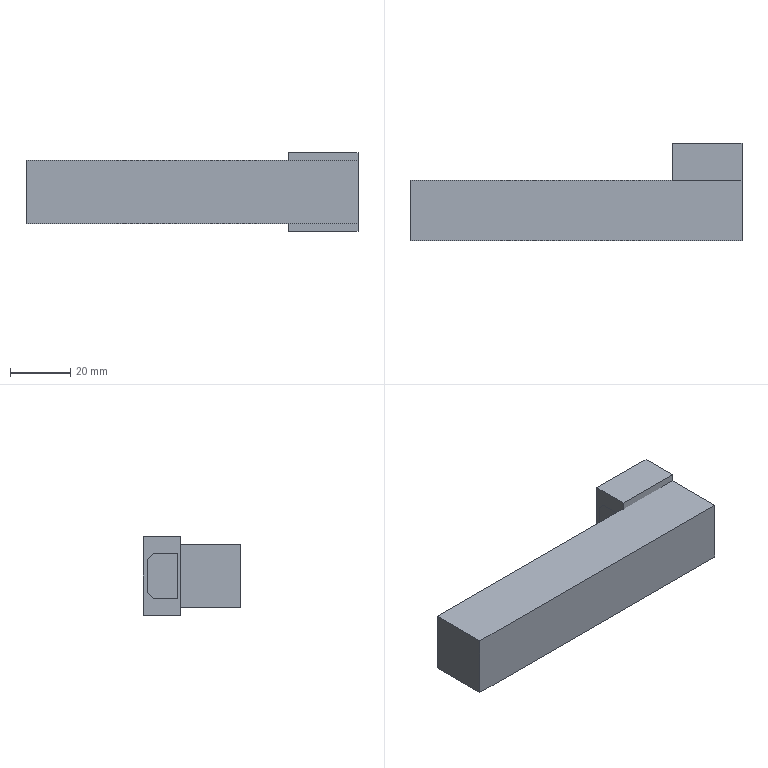NC program | NX | posted with a generic post | part box 110 x 32.2 x 26 mm
Lines 2299 to 4081 of 5595:
(PLANAR_MILL_2_COPY , TOOL : D4J)
N4560 T04 M6
N4562 G54
N4564 G17 G0 G90 X-42.552 Y0.455 S3500 M3
N4566 G43 Z20. H4
N4568 Z-2.067
N4570 G94 G1 Z-4.067 F400.
N4572 G41 X-42.5 Y0.75 D4
N4574 G3 X-43. Y1.25 R0.5
N4576 X-44.25 Y0. R1.25
N4578 X-43. Y-1.25 R1.25
N4580 G1 X22.
N4582 G3 X23.25 Y0. R1.25
N4584 X22. Y1.25 R1.25
N4586 G1 X-43.
N4588 G3 X-43.5 Y0.75 R0.5
N4590 G40
N4592 G1 X-43.448 Y0.455
N4594 X-42.552
N4596 G41 X-42.5 Y0.75
N4598 G3 X-43. Y1.25 R0.5
N4600 X-44.25 Y0. R1.25
N4602 X-43. Y-1.25 R1.25
N4604 G1 X22.
N4606 G3 X23.25 Y0. R1.25
N4608 X22. Y1.25 R1.25
N4610 G1 X-43.
N4612 G3 X-43.5 Y0.75 R0.5
N4614 G1 Y0.559
N4616 G40
N4618 X-43.448 Y0.264
N4620 Z-2.067
N4622 G0 Z20.
N4624 X-42.552 Y0.455
N4626 Z-6.133
N4628 G1 Z-8.133
N4630 G41 X-42.5 Y0.75
N4632 G3 X-43. Y1.25 R0.5
N4634 X-44.25 Y0. R1.25
N4636 X-43. Y-1.25 R1.25
N4638 G1 X22.
N4640 G3 X23.25 Y0. R1.25
N4642 X22. Y1.25 R1.25
N4644 G1 X-43.
N4646 G3 X-43.5 Y0.75 R0.5
N4648 G40
N4650 G1 X-43.448 Y0.455
N4652 X-42.552
N4654 G41 X-42.5 Y0.75
N4656 G3 X-43. Y1.25 R0.5
N4658 X-44.25 Y0. R1.25
N4660 X-43. Y-1.25 R1.25
N4662 G1 X22.
N4664 G3 X23.25 Y0. R1.25
N4666 X22. Y1.25 R1.25
N4668 G1 X-43.
N4670 G3 X-43.5 Y0.75 R0.5
N4672 G1 Y0.559
N4674 G40
N4676 X-43.448 Y0.264
N4678 Z-6.133
N4680 G0 Z20.
N4682 X-42.552 Y0.455
N4684 Z-10.2
N4686 G1 Z-12.2
N4688 G41 X-42.5 Y0.75
N4690 G3 X-43. Y1.25 R0.5
N4692 X-44.25 Y0. R1.25
N4694 X-43. Y-1.25 R1.25
N4696 G1 X22.
N4698 G3 X23.25 Y0. R1.25
N4700 X22. Y1.25 R1.25
N4702 G1 X-43.
N4704 G3 X-43.5 Y0.75 R0.5
N4706 G40
N4708 G1 X-43.448 Y0.455
N4710 X-42.552
N4712 G41 X-42.5 Y0.75
N4714 G3 X-43. Y1.25 R0.5
N4716 X-44.25 Y0. R1.25
N4718 X-43. Y-1.25 R1.25
N4720 G1 X22.
N4722 G3 X23.25 Y0. R1.25
N4724 X22. Y1.25 R1.25
N4726 G1 X-43.
N4728 G3 X-43.5 Y0.75 R0.5
N4730 G1 Y0.559
N4732 G40
N4734 X-43.448 Y0.264
N4736 Z-10.2
N4738 G0 Z20.
(FLOOR_WALL_1_COPY , TOOL : D4J)
N4740 X41. Y-11.44
N4742 Z-5.
N4744 G1 Z-7.
N4746 Y-6.44
N4748 X37.03
N4750 Y6.44
N4752 X44.97
N4754 Y-6.44
N4756 X41.
N4758 Y-3.44
N4760 X40.03
N4762 Y3.44
N4764 X41.97
N4766 Y-3.44
N4768 X41.
N4770 X40.03
N4772 Y-3.41
N4774 X38.03
N4776 Y-11.47
N4778 Z-5.
N4780 G0 Z20.
(PLANAR_MILL_3 , TOOL : D4J)
N4782 X37.174 Y12.425
N4784 Z-4.
N4786 G1 Z-7.
N4788 G41 X37. Y11.44
N4790 Y7.44
N4792 Y-7.44
N4794 Y-11.44
N4796 G40
N4798 X37.174 Y-12.425
N4800 Z-4.
N4802 G0 Z20.
N4804 X44.826
N4806 Z-4.
N4808 G1 Z-7.
N4810 G41 X45. Y-11.44
N4812 Y-7.44
N4814 Y7.44
N4816 Y11.44
N4818 G40
N4820 X44.826 Y12.425
N4822 Z-4.
N4824 G0 Z20.
N4826 M5
(PLANAR_MILL_COPY , TOOL : D16C)
N4828 T01 M6
N4830 G53
N4832 G17 G0 G90 X66. Y-0.06 S2300 M3
N4834 G43 Z20. H1
N4836 Z3.
N4838 G94 G1 Z0. F800.
N4840 X50.
N4842 X-48.06
N4844 X-64.06
N4846 Z3.
N4848 G0 Z20.
N4850 M5
(PLANAR_MILL_4 , TOOL : D4C)
N4852 T03 M6
N4854 G53
N4856 G17 G0 G90 X40.207 Y-0.973 S3500 M3
N4858 G43 Z20. H3
N4860 Z0.2
N4862 G94 G1 X40.724 Y-1.252 Z0.192 F800.
N4864 X41.276 Z0.184
N4866 X41.892 Y-0.92 Z0.174
N4868 X42.243 Y-0.313 Z0.165
N4870 X42.222 Y0.387 Z0.155
N4872 X41.946 Y0.864 Z0.147
N4874 X41.276 Y1.252 Z0.136
N4876 X40.724 Z0.129
N4878 X40.054 Y0.864 Z0.118
N4880 X39.778 Y0.387 Z0.11
N4882 X39.757 Y-0.313 Z0.1
N4884 X40.108 Y-0.92 Z0.09
N4886 X40.724 Y-1.252 Z0.081
N4888 X41.276 Z0.073
N4890 X41.892 Y-0.92 Z0.063
N4892 X42.243 Y-0.313 Z0.053
N4894 X42.222 Y0.387 Z0.044
N4896 X41.946 Y0.864 Z0.036
N4898 X41.276 Y1.252 Z0.025
N4900 X40.724 Z0.017
N4902 X40.054 Y0.864 Z0.007
N4904 X39.778 Y0.387 Z-0.001
N4906 X39.757 Y-0.313 Z-0.011
N4908 X40.108 Y-0.92 Z-0.021
N4910 X40.724 Y-1.252 Z-0.03
N4912 X41.276 Z-0.038
N4914 X41.892 Y-0.92 Z-0.048
N4916 X42.243 Y-0.313 Z-0.058
N4918 X42.222 Y0.387 Z-0.067
N4920 X41.946 Y0.864 Z-0.075
N4922 X41.276 Y1.252 Z-0.086
N4924 X40.724 Z-0.094
N4926 X40.054 Y0.864 Z-0.104
N4928 X39.778 Y0.387 Z-0.112
N4930 X39.757 Y-0.313 Z-0.122
N4932 X40.108 Y-0.92 Z-0.132
N4934 X40.724 Y-1.252 Z-0.141
N4936 X41.276 Z-0.149
N4938 X41.892 Y-0.92 Z-0.159
N4940 X42.243 Y-0.313 Z-0.169
N4942 X42.222 Y0.387 Z-0.179
N4944 X41.946 Y0.864 Z-0.186
N4946 X41.276 Y1.252 Z-0.197
N4948 X40.724 Z-0.205
N4950 X40.054 Y0.864 Z-0.216
N4952 X39.778 Y0.387 Z-0.223
N4954 X39.757 Y-0.313 Z-0.233
N4956 X40.108 Y-0.92 Z-0.243
N4958 X40.724 Y-1.252 Z-0.253
N4960 X41.276 Z-0.26
N4962 X41.892 Y-0.92 Z-0.27
N4964 X42.243 Y-0.313 Z-0.28
N4966 X42.222 Y0.387 Z-0.29
N4968 X41.946 Y0.864 Z-0.297
N4970 X41.276 Y1.252 Z-0.308
N4972 X40.724 Z-0.316
N4974 X40.054 Y0.864 Z-0.327
N4976 X39.778 Y0.387 Z-0.334
N4978 X39.757 Y-0.313 Z-0.344
N4980 X40.108 Y-0.92 Z-0.354
N4982 X40.724 Y-1.252 Z-0.364
N4984 X41.276 Z-0.371
N4986 X41.892 Y-0.92 Z-0.381
N4988 X42.243 Y-0.313 Z-0.391
N4990 X42.222 Y0.387 Z-0.401
N4992 X41.946 Y0.864 Z-0.408
N4994 X41.276 Y1.252 Z-0.419
N4996 X40.724 Z-0.427
N4998 X40.054 Y0.864 Z-0.438
N5000 X39.778 Y0.387 Z-0.445
N5002 X39.757 Y-0.313 Z-0.455
N5004 X40.108 Y-0.92 Z-0.465
N5006 X40.724 Y-1.252 Z-0.475
N5008 X41.276 Z-0.482
N5010 X41.892 Y-0.92 Z-0.492
N5012 X42.243 Y-0.313 Z-0.502
N5014 X42.222 Y0.387 Z-0.512
N5016 X41.946 Y0.864 Z-0.519
N5018 X41.276 Y1.252 Z-0.53
N5020 X40.724 Z-0.538
N5022 X40.054 Y0.864 Z-0.549
N5024 X39.778 Y0.387 Z-0.557
N5026 X39.757 Y-0.313 Z-0.566
N5028 X40.108 Y-0.92 Z-0.576
N5030 X40.724 Y-1.252 Z-0.586
N5032 X41.276 Z-0.594
N5034 X41.892 Y-0.92 Z-0.603
N5036 X42.243 Y-0.313 Z-0.613
N5038 X42.222 Y0.387 Z-0.623
N5040 X41.946 Y0.864 Z-0.631
N5042 X41.276 Y1.252 Z-0.641
N5044 X40.724 Z-0.649
N5046 X40.054 Y0.864 Z-0.66
N5048 X39.778 Y0.387 Z-0.668
N5050 X39.757 Y-0.313 Z-0.677
N5052 X40.108 Y-0.92 Z-0.687
N5054 X40.724 Y-1.252 Z-0.697
N5056 X41.276 Z-0.705
N5058 X41.892 Y-0.92 Z-0.714
N5060 X42.243 Y-0.313 Z-0.724
N5062 X42.222 Y0.387 Z-0.734
N5064 X41.946 Y0.864 Z-0.742
N5066 X41.276 Y1.252 Z-0.752
N5068 X40.724 Z-0.76
N5070 X40.054 Y0.864 Z-0.771
N5072 X39.778 Y0.387 Z-0.779
N5074 X39.757 Y-0.313 Z-0.788
N5076 X40.108 Y-0.92 Z-0.798
N5078 X40.724 Y-1.252 Z-0.808
N5080 X41.276 Z-0.816
N5082 X41.892 Y-0.92 Z-0.826
N5084 X42.243 Y-0.313 Z-0.835
N5086 X42.222 Y0.387 Z-0.845
N5088 X41.946 Y0.864 Z-0.853
N5090 X41.276 Y1.252 Z-0.864
N5092 X40.724 Z-0.871
N5094 X40.054 Y0.864 Z-0.882
N5096 X39.778 Y0.387 Z-0.89
N5098 X39.757 Y-0.313 Z-0.9
N5100 X40.108 Y-0.92 Z-0.909
N5102 X40.724 Y-1.252 Z-0.919
N5104 X41.276 Z-0.927
N5106 X41.892 Y-0.92 Z-0.937
N5108 X42.243 Y-0.313 Z-0.946
N5110 X42.222 Y0.387 Z-0.956
N5112 X41.946 Y0.864 Z-0.964
N5114 X41.276 Y1.252 Z-0.975
N5116 X40.724 Z-0.982
N5118 X40.054 Y0.864 Z-0.993
N5120 X39.778 Y0.387 Z-1.001
N5122 X39.757 Y-0.313 Z-1.011
N5124 X40.108 Y-0.92 Z-1.02
N5126 X40.724 Y-1.252 Z-1.03
N5128 X41.276 Z-1.038
N5130 X41.892 Y-0.92 Z-1.048
N5132 X42.243 Y-0.313 Z-1.057
N5134 X42.222 Y0.387 Z-1.067
N5136 X41.946 Y0.864 Z-1.075
N5138 X41.276 Y1.252 Z-1.086
N5140 X40.724 Z-1.093
N5142 X40.054 Y0.864 Z-1.104
N5144 X39.778 Y0.387 Z-1.112
N5146 X39.757 Y-0.313 Z-1.122
N5148 X40.108 Y-0.92 Z-1.132
N5150 X40.724 Y-1.252 Z-1.141
N5152 X41.276 Z-1.149
N5154 X41.892 Y-0.92 Z-1.159
N5156 X42.243 Y-0.313 Z-1.169
N5158 X42.222 Y0.387 Z-1.178
N5160 X41.946 Y0.864 Z-1.186
N5162 X41.276 Y1.252 Z-1.197
N5164 X40.724 Z-1.205
N5166 X40.054 Y0.864 Z-1.215
N5168 X39.778 Y0.387 Z-1.223
N5170 X39.757 Y-0.313 Z-1.233
N5172 X40.108 Y-0.92 Z-1.243
N5174 X40.724 Y-1.252 Z-1.252
N5176 X41.276 Z-1.26
N5178 X41.892 Y-0.92 Z-1.27
N5180 X42.243 Y-0.313 Z-1.28
N5182 X42.222 Y0.387 Z-1.289
N5184 X41.946 Y0.864 Z-1.297
N5186 X41.276 Y1.252 Z-1.308
N5188 X40.724 Z-1.316
N5190 X40.054 Y0.864 Z-1.326
N5192 X39.778 Y0.387 Z-1.334
N5194 X39.757 Y-0.313 Z-1.344
N5196 X40.108 Y-0.92 Z-1.354
N5198 X40.724 Y-1.252 Z-1.363
N5200 X41.276 Z-1.371
N5202 X41.892 Y-0.92 Z-1.381
N5204 X42.243 Y-0.313 Z-1.391
N5206 X42.222 Y0.387 Z-1.401
N5208 X41.946 Y0.864 Z-1.408
N5210 X41.276 Y1.252 Z-1.419
N5212 X40.724 Z-1.427
N5214 X40.054 Y0.864 Z-1.438
N5216 X39.778 Y0.387 Z-1.445
N5218 X39.757 Y-0.313 Z-1.455
N5220 X40.108 Y-0.92 Z-1.465
N5222 X40.724 Y-1.252 Z-1.475
N5224 X41.276 Z-1.482
N5226 X41.892 Y-0.92 Z-1.492
N5228 X42.243 Y-0.313 Z-1.502
N5230 X42.222 Y0.387 Z-1.512
N5232 X41.946 Y0.864 Z-1.519
N5234 X41.276 Y1.252 Z-1.53
N5236 X40.724 Z-1.538
N5238 X40.054 Y0.864 Z-1.549
N5240 X39.778 Y0.387 Z-1.556
N5242 X39.757 Y-0.313 Z-1.566
N5244 X40.108 Y-0.92 Z-1.576
N5246 X40.724 Y-1.252 Z-1.586
N5248 X41.276 Z-1.593
N5250 X41.892 Y-0.92 Z-1.603
N5252 X42.243 Y-0.313 Z-1.613
N5254 X42.222 Y0.387 Z-1.623
N5256 X41.946 Y0.864 Z-1.63
N5258 X41.276 Y1.252 Z-1.641
N5260 X40.724 Z-1.649
N5262 X40.054 Y0.864 Z-1.66
N5264 X39.778 Y0.387 Z-1.667
N5266 X39.757 Y-0.313 Z-1.677
N5268 X40.108 Y-0.92 Z-1.687
N5270 X40.724 Y-1.252 Z-1.697
N5272 X41.276 Z-1.704
N5274 X41.892 Y-0.92 Z-1.714
N5276 X42.243 Y-0.313 Z-1.724
N5278 X42.222 Y0.387 Z-1.734
N5280 X41.946 Y0.864 Z-1.742
N5282 X41.276 Y1.252 Z-1.752
N5284 X40.724 Z-1.76
N5286 X40.054 Y0.864 Z-1.771
N5288 X39.778 Y0.387 Z-1.779
N5290 X39.757 Y-0.313 Z-1.788
N5292 X40.108 Y-0.92 Z-1.798
N5294 X40.724 Y-1.252 Z-1.808
N5296 X41.276 Z-1.816
N5298 X41.892 Y-0.92 Z-1.825
N5300 X42.243 Y-0.313 Z-1.835
N5302 X42.222 Y0.387 Z-1.845
N5304 X41.946 Y0.864 Z-1.853
N5306 X41.276 Y1.252 Z-1.863
N5308 X40.724 Z-1.871
N5310 X40.054 Y0.864 Z-1.882
N5312 X39.778 Y0.387 Z-1.89
N5314 X39.757 Y-0.313 Z-1.899
N5316 X40.108 Y-0.92 Z-1.909
N5318 X40.724 Y-1.252 Z-1.919
N5320 X41.276 Z-1.927
N5322 X41.892 Y-0.92 Z-1.936
N5324 X42.243 Y-0.313 Z-1.946
N5326 X42.222 Y0.387 Z-1.956
N5328 X41.946 Y0.864 Z-1.964
N5330 X41.276 Y1.252 Z-1.974
N5332 X40.724 Z-1.982
N5334 X40.054 Y0.864 Z-1.993
N5336 X39.778 Y0.387 Z-2.001
N5338 X39.757 Y-0.313 Z-2.01
N5340 X40.108 Y-0.92 Z-2.02
N5342 X40.724 Y-1.252 Z-2.03
N5344 X41.276 Z-2.038
N5346 X41.892 Y-0.92 Z-2.048
N5348 X42.243 Y-0.313 Z-2.057
N5350 X42.222 Y0.387 Z-2.067
N5352 X41.946 Y0.864 Z-2.075
N5354 X41.276 Y1.252 Z-2.086
N5356 X40.724 Z-2.093
N5358 X40.054 Y0.864 Z-2.104
N5360 X39.778 Y0.387 Z-2.112
N5362 X39.757 Y-0.313 Z-2.122
N5364 X40.108 Y-0.92 Z-2.131
N5366 X40.724 Y-1.252 Z-2.141
N5368 X41.276 Z-2.149
N5370 X41.892 Y-0.92 Z-2.159
N5372 X42.243 Y-0.313 Z-2.168
N5374 X42.222 Y0.387 Z-2.178
N5376 X41.946 Y0.864 Z-2.186
N5378 X41.276 Y1.252 Z-2.197
N5380 X40.724 Z-2.204
N5382 X40.054 Y0.864 Z-2.215
N5384 X39.778 Y0.387 Z-2.223
N5386 X39.757 Y-0.313 Z-2.233
N5388 X40.108 Y-0.92 Z-2.242
N5390 X40.724 Y-1.252 Z-2.252
N5392 X41.276 Z-2.26
N5394 X41.892 Y-0.92 Z-2.27
N5396 X42.243 Y-0.313 Z-2.279
N5398 X42.222 Y0.387 Z-2.289
N5400 X41.946 Y0.864 Z-2.297
N5402 X41.276 Y1.252 Z-2.308
N5404 X40.724 Z-2.315
N5406 X40.054 Y0.864 Z-2.326
N5408 X39.778 Y0.387 Z-2.334
N5410 X39.757 Y-0.313 Z-2.344
N5412 X40.108 Y-0.92 Z-2.354
N5414 X40.724 Y-1.252 Z-2.363
N5416 X41.276 Z-2.371
N5418 X41.892 Y-0.92 Z-2.381
N5420 X42.243 Y-0.313 Z-2.391
N5422 X42.222 Y0.387 Z-2.4
N5424 X41.946 Y0.864 Z-2.408
N5426 X41.276 Y1.252 Z-2.419
N5428 X40.724 Z-2.427
N5430 X40.054 Y0.864 Z-2.437
N5432 X39.778 Y0.387 Z-2.445
N5434 X39.757 Y-0.313 Z-2.455
N5436 X40.108 Y-0.92 Z-2.465
N5438 X40.724 Y-1.252 Z-2.474
N5440 X41.276 Z-2.482
N5442 X41.892 Y-0.92 Z-2.492
N5444 X42.243 Y-0.313 Z-2.502
N5446 X42.222 Y0.387 Z-2.511
N5448 X41.946 Y0.864 Z-2.519
N5450 X41.276 Y1.252 Z-2.53
N5452 X40.724 Z-2.538
N5454 X40.054 Y0.864 Z-2.548
N5456 X39.778 Y0.387 Z-2.556
N5458 X39.757 Y-0.313 Z-2.566
N5460 X40.108 Y-0.92 Z-2.576
N5462 X40.724 Y-1.252 Z-2.586
N5464 X41.276 Z-2.593
N5466 X41.892 Y-0.92 Z-2.603
N5468 X42.243 Y-0.313 Z-2.613
N5470 X42.222 Y0.387 Z-2.623
N5472 X41.946 Y0.864 Z-2.63
N5474 X41.276 Y1.252 Z-2.641
N5476 X40.724 Z-2.649
N5478 X40.054 Y0.864 Z-2.66
N5480 X39.778 Y0.387 Z-2.667
N5482 X39.757 Y-0.313 Z-2.677
N5484 X40.108 Y-0.92 Z-2.687
N5486 X40.724 Y-1.252 Z-2.697
N5488 X41.276 Z-2.704
N5490 X41.892 Y-0.92 Z-2.714
N5492 X42.243 Y-0.313 Z-2.724
N5494 X42.222 Y0.387 Z-2.734
N5496 X41.946 Y0.864 Z-2.741
N5498 X41.276 Y1.252 Z-2.752
N5500 X40.724 Z-2.76
N5502 X40.054 Y0.864 Z-2.771
N5504 X39.778 Y0.387 Z-2.778
N5506 X39.757 Y-0.313 Z-2.788
N5508 X40.108 Y-0.92 Z-2.798
N5510 X40.724 Y-1.252 Z-2.808
N5512 X41.276 Z-2.815
N5514 X41.892 Y-0.92 Z-2.825
N5516 X42.243 Y-0.313 Z-2.835
N5518 X42.222 Y0.387 Z-2.845
N5520 X41.946 Y0.864 Z-2.852
N5522 X41.276 Y1.252 Z-2.863
N5524 X40.724 Z-2.871
N5526 X40.054 Y0.864 Z-2.882
N5528 X39.778 Y0.387 Z-2.889
N5530 X39.757 Y-0.313 Z-2.899
N5532 X40.108 Y-0.92 Z-2.909
N5534 X40.724 Y-1.252 Z-2.919
N5536 X41.276 Z-2.926
N5538 X41.892 Y-0.92 Z-2.936
N5540 X42.243 Y-0.313 Z-2.946
N5542 X42.222 Y0.387 Z-2.956
N5544 X41.946 Y0.864 Z-2.964
N5546 X41.276 Y1.252 Z-2.974
N5548 X40.724 Z-2.982
N5550 X40.054 Y0.864 Z-2.993
N5552 X39.778 Y0.387 Z-3.001
N5554 X39.757 Y-0.313 Z-3.01
N5556 X40.108 Y-0.92 Z-3.02
N5558 X40.724 Y-1.252 Z-3.03
N5560 X41.276 Z-3.038
N5562 X41.892 Y-0.92 Z-3.047
N5564 X42.243 Y-0.313 Z-3.057
N5566 X42.222 Y0.387 Z-3.067
N5568 X41.946 Y0.864 Z-3.075
N5570 X41.276 Y1.252 Z-3.085
N5572 X40.724 Z-3.093
N5574 X40.054 Y0.864 Z-3.104
N5576 X39.778 Y0.387 Z-3.112
N5578 X39.757 Y-0.313 Z-3.121
N5580 X40.108 Y-0.92 Z-3.131
N5582 X40.724 Y-1.252 Z-3.141
N5584 X41.276 Z-3.149
N5586 X41.892 Y-0.92 Z-3.158
N5588 X42.243 Y-0.313 Z-3.168
N5590 X42.222 Y0.387 Z-3.178
N5592 X41.946 Y0.864 Z-3.186
N5594 X41.276 Y1.252 Z-3.197
N5596 X40.724 Z-3.204
N5598 X40.054 Y0.864 Z-3.215
N5600 X39.778 Y0.387 Z-3.223
N5602 X39.757 Y-0.313 Z-3.232
N5604 X40.108 Y-0.92 Z-3.242
N5606 X40.724 Y-1.252 Z-3.252
N5608 X41.276 Z-3.26
N5610 X41.892 Y-0.92 Z-3.27
N5612 X42.243 Y-0.313 Z-3.279
N5614 X42.222 Y0.387 Z-3.289
N5616 X41.946 Y0.864 Z-3.297
N5618 X41.276 Y1.252 Z-3.308
N5620 X40.724 Z-3.315
N5622 X40.054 Y0.864 Z-3.326
N5624 X39.778 Y0.387 Z-3.334
N5626 X39.757 Y-0.313 Z-3.344
N5628 X40.108 Y-0.92 Z-3.353
N5630 X40.724 Y-1.252 Z-3.363
N5632 X41.276 Z-3.371
N5634 X41.892 Y-0.92 Z-3.381
N5636 X42.243 Y-0.313 Z-3.39
N5638 X42.222 Y0.387 Z-3.4
N5640 X41.946 Y0.864 Z-3.408
N5642 X41.276 Y1.252 Z-3.419
N5644 X40.724 Z-3.426
N5646 X40.054 Y0.864 Z-3.437
N5648 X39.778 Y0.387 Z-3.445
N5650 X39.757 Y-0.313 Z-3.455
N5652 X40.108 Y-0.92 Z-3.464
N5654 X40.724 Y-1.252 Z-3.474
N5656 X41.276 Z-3.482
N5658 X41.892 Y-0.92 Z-3.492
N5660 X42.243 Y-0.313 Z-3.501
N5662 X42.222 Y0.387 Z-3.511
N5664 X41.946 Y0.864 Z-3.519
N5666 X41.276 Y1.252 Z-3.53
N5668 X40.724 Z-3.537
N5670 X40.054 Y0.864 Z-3.548
N5672 X39.778 Y0.387 Z-3.556
N5674 X39.757 Y-0.313 Z-3.566
N5676 X40.108 Y-0.92 Z-3.576
N5678 X40.724 Y-1.252 Z-3.585
N5680 X41.276 Z-3.593
N5682 X41.892 Y-0.92 Z-3.603
N5684 X42.243 Y-0.313 Z-3.613
N5686 X42.222 Y0.387 Z-3.622
N5688 X41.946 Y0.864 Z-3.63
N5690 X41.276 Y1.252 Z-3.641
N5692 X40.724 Z-3.649
N5694 X40.054 Y0.864 Z-3.659
N5696 X39.778 Y0.387 Z-3.667
N5698 X39.757 Y-0.313 Z-3.677
N5700 X40.108 Y-0.92 Z-3.687
N5702 X40.724 Y-1.252 Z-3.696
N5704 X41.276 Z-3.704
N5706 X41.892 Y-0.92 Z-3.714
N5708 X42.243 Y-0.313 Z-3.724
N5710 X42.222 Y0.387 Z-3.733
N5712 X41.946 Y0.864 Z-3.741
N5714 X41.276 Y1.252 Z-3.752
N5716 X40.724 Z-3.76
N5718 X40.054 Y0.864 Z-3.77
N5720 X39.778 Y0.387 Z-3.778
N5722 X39.757 Y-0.313 Z-3.788
N5724 X40.108 Y-0.92 Z-3.798
N5726 X40.724 Y-1.252 Z-3.808
N5728 X41.276 Z-3.815
N5730 X41.892 Y-0.92 Z-3.825
N5732 X42.243 Y-0.313 Z-3.835
N5734 X42.222 Y0.387 Z-3.845
N5736 X41.946 Y0.864 Z-3.852
N5738 X41.276 Y1.252 Z-3.863
N5740 X40.724 Z-3.871
N5742 X40.054 Y0.864 Z-3.882
N5744 X39.778 Y0.387 Z-3.889
N5746 X39.757 Y-0.313 Z-3.899
N5748 X40.108 Y-0.92 Z-3.909
N5750 X40.724 Y-1.252 Z-3.919
N5752 X41.276 Z-3.926
N5754 X41.892 Y-0.92 Z-3.936
N5756 X42.243 Y-0.313 Z-3.946
N5758 X42.222 Y0.387 Z-3.956
N5760 X41.946 Y0.864 Z-3.963
N5762 X41.276 Y1.252 Z-3.974
N5764 X40.724 Z-3.982
N5766 X40.054 Y0.864 Z-3.993
N5768 X39.778 Y0.387 Z-4.
N5770 X39.757 Y-0.313 Z-4.01
N5772 X40.108 Y-0.92 Z-4.02
N5774 X40.724 Y-1.252 Z-4.03
N5776 X41.276 Z-4.037
N5778 X41.892 Y-0.92 Z-4.047
N5780 X42.243 Y-0.313 Z-4.057
N5782 X42.222 Y0.387 Z-4.067
N5784 X41.946 Y0.864 Z-4.074
N5786 X41.276 Y1.252 Z-4.085
N5788 X40.724 Z-4.093
N5790 X40.054 Y0.864 Z-4.104
N5792 X39.778 Y0.387 Z-4.111
N5794 X39.757 Y-0.313 Z-4.121
N5796 X40.108 Y-0.92 Z-4.131
N5798 X40.724 Y-1.252 Z-4.141
N5800 X41.276 Z-4.148
N5802 X41.892 Y-0.92 Z-4.158
N5804 X42.243 Y-0.313 Z-4.168
N5806 X42.222 Y0.387 Z-4.178
N5808 X41.946 Y0.864 Z-4.186
N5810 X41.276 Y1.252 Z-4.196
N5812 X40.724 Z-4.204
N5814 X40.054 Y0.864 Z-4.215
N5816 X39.778 Y0.387 Z-4.223
N5818 X39.757 Y-0.313 Z-4.232
N5820 X40.108 Y-0.92 Z-4.242
N5822 X40.724 Y-1.252 Z-4.252
N5824 X41.276 Z-4.26
N5826 X41.892 Y-0.92 Z-4.269
N5828 X42.243 Y-0.313 Z-4.279
N5830 X42.222 Y0.387 Z-4.289
N5832 X41.946 Y0.864 Z-4.297
N5834 X41.276 Y1.252 Z-4.307
N5836 X40.724 Z-4.315
N5838 X40.054 Y0.864 Z-4.326
N5840 X39.778 Y0.387 Z-4.334
N5842 X39.757 Y-0.313 Z-4.343
N5844 X40.108 Y-0.92 Z-4.353
N5846 X40.724 Y-1.252 Z-4.363
N5848 X41.276 Z-4.371
N5850 X41.892 Y-0.92 Z-4.38
N5852 X42.243 Y-0.313 Z-4.39
N5854 X42.222 Y0.387 Z-4.4
N5856 X41.946 Y0.864 Z-4.408
N5858 X41.276 Y1.252 Z-4.419
N5860 X40.724 Z-4.426
N5862 X40.054 Y0.864 Z-4.437
N5864 X39.778 Y0.387 Z-4.445
N5866 X39.757 Y-0.313 Z-4.454
N5868 X40.108 Y-0.92 Z-4.464
N5870 X40.724 Y-1.252 Z-4.474
N5872 X41.276 Z-4.482
N5874 X41.892 Y-0.92 Z-4.492
N5876 X42.243 Y-0.313 Z-4.501
N5878 X42.222 Y0.387 Z-4.511
N5880 X41.946 Y0.864 Z-4.519
N5882 X41.276 Y1.252 Z-4.53
N5884 X40.724 Z-4.537
N5886 X40.054 Y0.864 Z-4.548
N5888 X39.778 Y0.387 Z-4.556
N5890 X39.757 Y-0.313 Z-4.566
N5892 X40.108 Y-0.92 Z-4.575
N5894 X40.724 Y-1.252 Z-4.585
N5896 X41.276 Z-4.593
N5898 X41.892 Y-0.92 Z-4.603
N5900 X42.243 Y-0.313 Z-4.612
N5902 X42.222 Y0.387 Z-4.622
N5904 X41.946 Y0.864 Z-4.63
N5906 X41.276 Y1.252 Z-4.641
N5908 X40.724 Z-4.648
N5910 X40.054 Y0.864 Z-4.659
N5912 X39.778 Y0.387 Z-4.667
N5914 X39.757 Y-0.313 Z-4.677
N5916 X40.108 Y-0.92 Z-4.686
N5918 X40.724 Y-1.252 Z-4.696
N5920 X41.276 Z-4.704
N5922 X41.892 Y-0.92 Z-4.714
N5924 X42.243 Y-0.313 Z-4.723
N5926 X42.222 Y0.387 Z-4.733
N5928 X41.946 Y0.864 Z-4.741
N5930 X41.276 Y1.252 Z-4.752
N5932 X40.724 Z-4.759
N5934 X40.054 Y0.864 Z-4.77
N5936 X39.778 Y0.387 Z-4.778
N5938 X39.757 Y-0.313 Z-4.788
N5940 X40.108 Y-0.92 Z-4.798
N5942 X40.724 Y-1.252 Z-4.807
N5944 X41.276 Z-4.815
N5946 X41.892 Y-0.92 Z-4.825
N5948 X42.243 Y-0.313 Z-4.835
N5950 X42.222 Y0.387 Z-4.844
N5952 X41.946 Y0.864 Z-4.852
N5954 X41.276 Y1.252 Z-4.863
N5956 X40.724 Z-4.871
N5958 X40.054 Y0.864 Z-4.881
N5960 X39.778 Y0.387 Z-4.889
N5962 X39.757 Y-0.313 Z-4.899
N5964 X40.108 Y-0.92 Z-4.909
N5966 X40.724 Y-1.252 Z-4.918
N5968 X41.276 Z-4.926
N5970 X41.892 Y-0.92 Z-4.936
N5972 X42.243 Y-0.313 Z-4.946
N5974 X42.222 Y0.387 Z-4.955
N5976 X41.946 Y0.864 Z-4.963
N5978 X41.276 Y1.252 Z-4.974
N5980 X40.724 Z-4.982
N5982 X40.054 Y0.864 Z-4.992
N5984 X39.778 Y0.387 Z-5.
N5986 X39.757 Y-0.313 Z-5.01
N5988 X40.108 Y-0.92 Z-5.02
N5990 X40.724 Y-1.252 Z-5.03
N5992 X41.276 Z-5.037
N5994 X41.892 Y-0.92 Z-5.047
N5996 X42.243 Y-0.313 Z-5.057
N5998 X42.222 Y0.387 Z-5.067
N6000 X41.946 Y0.864 Z-5.074
N6002 X41.276 Y1.252 Z-5.085
N6004 X40.724 Z-5.093
N6006 X40.054 Y0.864 Z-5.104
N6008 X39.778 Y0.387 Z-5.111
N6010 X39.757 Y-0.313 Z-5.121
N6012 X40.108 Y-0.92 Z-5.131
N6014 X40.724 Y-1.252 Z-5.141
N6016 X41.276 Z-5.148
N6018 X41.892 Y-0.92 Z-5.158
N6020 X42.243 Y-0.313 Z-5.168
N6022 X42.222 Y0.387 Z-5.178
N6024 X41.946 Y0.864 Z-5.185
N6026 X41.276 Y1.252 Z-5.196
N6028 X41. Z-5.2
N6030 G3 X39.749 Y0. R1.252
N6032 X41. Y1.252 R-1.252
N6034 G1 Z-5.
N6036 G0 Z20.
N6038 M5
(PLANAR_MILL_5 , TOOL : D4DJ)
N6040 T05 M6
N6042 G53
N6044 G17 G0 G90 X23. Y0.75 S3000 M3
N6046 G43 Z20. H5
N6048 Z1.
N6050 G94 G1 Z-1. F1000.
N6052 Y1.25
N6054 G3 X22. Y2.25 R1.
N6056 G1 X-43.
N6058 G3 X-45.25 Y0. R2.25
N6060 X-43. Y-2.25 R2.25
N6062 G1 X22.
N6064 G3 X24.25 Y0. R2.25
N6066 X22. Y2.25 R2.25
N6068 X21. Y1.25 R1.
N6070 G1 Z1.
N6072 G0 Z20.
N6074 X40. Y-0.752
N6076 Z1.
N6078 G1 Z-1.
N6080 Y-1.252
N6082 G3 X41. Y-2.252 R1.
N6084 X43.252 Y0. R2.252
N6086 X41. Y-2.252 R-2.252
N6088 X42. Y-1.252 R1.
N6090 G1 Y-0.752
N6092 Z1.
N6094 G0 Z20.
(PLANAR_MILL_5_COPY , TOOL : D4DJ)
N6096 X52. Y-6.44
N6098 Z1.
N6100 G1 Z-1.
N6102 G3 X51. Y-7.44 R1.
N6104 G2 X50. Y-8.44 R1.
N6106 G1 X-48.06
N6108 G2 X-48.767 Y-8.147 R1.
N6110 G1 X-50.707 Y-6.207
N6112 G2 X-51. Y-5.5 R1.
N6114 G1 Y5.5
N6116 G2 X-50.707 Y6.207 R1.
N6118 G1 X-48.767 Y8.147
N6120 G2 X-48.06 Y8.44 R1.
N6122 G1 X50.
N6124 G2 X51. Y7.44 R1.
N6126 G1 Y-7.44
N6128 G3 X52. Y-8.44 R1.
N6130 G1 Z1.
N6132 G0 Z20.
N6134 M5
(PLANAR_MILL_6 , TOOL : D16C)
N6136 T01 M6
N6138 G54
N6140 G17 G0 G90 X23.5 Y-1. S2300 M3
N6142 G43 Z20. H1
N6144 Z3.
N6146 G94 G1 Z0. F600.
N6148 X7.5
N6150 X-7.5
N6152 X-23.5
N6154 Z3.
N6156 G0 Z20.
(ADAPTIVE_MILLING_1 , TOOL : D16C)
N6158 X25.701 Y14.017 S3500
N6160 Z-16.
N6162 G1 X25.572 Y13.941 Z-16.937 F1500.
N6164 X25.442 Y13.866 Z-17.308
N6166 X25.312 Y13.791 Z-17.58
N6168 X25.182 Y13.716 Z-17.8
N6170 X25.053 Y13.64 Z-17.984
N6172 X24.923 Y13.565 Z-18.142
N6174 X24.793 Y13.49 Z-18.28
N6176 X24.663 Y13.414 Z-18.4
N6178 X24.534 Y13.339 Z-18.505
N6180 X24.404 Y13.264 Z-18.598
N6182 X24.274 Y13.189 Z-18.679
N6184 X24.144 Y13.113 Z-18.75
N6186 X24.015 Y13.038 Z-18.81
N6188 X23.885 Y12.963 Z-18.862
N6190 X23.755 Y12.888 Z-18.905
N6192 X23.625 Y12.812 Z-18.939
N6194 X23.496 Y12.737 Z-18.966
N6196 X23.366 Y12.662 Z-18.985
N6198 X23.236 Y12.586 Z-18.996
N6200 X23.106 Y12.511 Z-19.
N6202 X20.932 Y11.25
N6204 G3 X20.154 Y9.558 R1.616
N6206 G2 X20.587 Y6.395 R12.497
N6208 X20.675 Y-4.516 R227.945
N6210 X17.038 Y-11.021 R8.943
N6212 X11.305 Y-13.391 R13.202
N6214 X5.03 Y-13.862 R39.811
N6216 X-11.22 Y-13.882 R893.255
N6218 X-17.72 Y-10.352 R8.92
N6220 X-20.183 Y-4.531 R13.112
N6222 X-20.662 Y1.782 R39.494
N6224 X-20.615 Y5.004 R26.234
N6226 X-16.75 Y11.211 R9.081
N6228 X-10.952 Y13.446 R13.654
N6230 X-4.522 Y13.869 R44.518
N6232 X10.89 Y13.887 R908.336
N6234 X17.333 Y10.399 R8.956
N6236 X19.838 Y4.636 R13.087
N6238 X20.355 Y-1.635 R37.456
N6240 X15.482 Y-10.823 R10.52
N6242 X9.25 Y-13.099 R15.678
N6244 X2.484 Y-13.559 R48.53
N6246 X-9.328 Y-13.581 R647.832
N6248 X-17.727 Y-8.531 R10.619
N6250 X-19.903 Y-2.422 R15.875
N6252 X-20.265 Y2.77 R27.224
N6254 X-15.482 Y10.79 R10.489
N6256 X-9.331 Y13.078 R15.536
N6258 X-2.604 Y13.557 R46.731
N6260 X9.021 Y13.579 R470.728
N6262 X17.411 Y8.504 R10.671
N6264 X19.617 Y2.24 R16.079
N6266 X19.772 Y-2.39 R15.803
N6268 X14.307 Y-10.534 R11.441
N6270 X7.754 Y-12.789 R17.309
N6272 X0.424 Y-13.259 R55.185
N6274 X-7.895 Y-13.267 R209.836
N6276 X-17.59 Y-7.136 R11.748
N6278 X-19.73 Y1.282 R17.546
N6280 X-14.601 Y10.293 R11.198
N6282 X-11.667 Y11.8 R16.552
N6284 G1 X-11.131 Y12.129
N6286 G2 X-8.565 Y12.931 R9.231
N6288 X2.366 Y13.289 R134.099
N6290 X7.728 Y13.255 R103.637
N6292 X17.216 Y7.222 R11.768
N6294 X19.241 Y-0.563 R14.922
N6296 X13.92 Y-9.812 R11.696
N6298 X9.721 Y-11.779 R16.539
N6300 G1 X9.131 Y-12.129
N6302 G2 X6.75 Y-12.902 R9.316
N6304 G1 X5.499 Y-13.
N6306 G2 X-6.213 Y-12.982 R869.141
N6308 X-14.742 Y-9.531 R12.672
N6310 X-19.028 Y0.004 R14.26
N6312 X-14.794 Y9.079 R11.396
N6314 G1 X-13.81 Y9.892
N6316 X-13.156 Y10.658
N6318 G2 X-11.131 Y12.129 R9.312
N6320 X-8.75 Y12.902 R9.316
N6322 G1 X-7.499 Y13.
N6324 X7.501
N6326 G2 X9.973 Y12.608 R9.319
N6328 X14.326 Y9.824 R11.906
N6330 X18.472 Y1.181 R13.654
N6332 X13.843 Y-8.861 R11.64
N6334 X11.294 Y-10.534 R31.864
N6336 G1 X10.201 Y-11.473
N6338 X9.594 Y-11.845
N6340 G3 X9.623 Y-14.591 R1.6
N6342 X10.785 Y-14.777 Z-18.962 R1.701
N6344 G1 X12.755 Y-14.523 Z-18.9
N6346 X15.598 Y-14.158 F15000.
N6348 G3 X16.525 Y-13.702 R1.604
N6350 G1 X17.433 Y-12.8
N6352 X18.327 Y-11.885
N6354 G3 X20.323 Y-9.147 R14.598
N6356 G1 X22.282 Y-5.674
N6358 G3 X23.552 Y-1.467 R10.091
N6360 X23.365 Y1.977 R12.707
N6362 G1 X22.529 Y6.31
N6364 G3 X20.009 Y11.642 R11.87
N6366 G1 X18.065 Y13.985
N6368 G3 X17.006 Y14.554 R1.602
N6370 G1 X14.35 Y14.842
N6372 X13.198 Y14.972 Z-18.936 F1500.
N6374 X12.045 Y15.087 Z-18.973
N6376 G3 X11.206 Y14.898 Z-19. R1.602
N6378 X11.133 Y12.127 R1.6
N6380 G2 X13.98 Y9.758 R9.314
N6382 X17.296 Y3.876 R15.158
N6384 X14.558 Y-7.092 R11.557
N6386 G3 X13.156 Y-8.657 R27.808
N6388 G1 X11.194 Y-10.619
N6390 G3 X12.198 Y-13.346 R1.6
N6392 X13.094 Y-13.162 Z-18.971 R1.762
N6394 G1 X15.175 Y-12.271 Z-18.9
N6396 X17.669 Y-11.203 F15000.
N6398 G3 X18.37 Y-10.619 R1.608
N6400 G1 X19.366 Y-9.131
N6402 X20.348 Y-7.633
N6404 G3 X22.389 Y-2.737 R16.864
N6406 G1 X22.57 Y-1.984
N6408 X22.741 Y-1.229
N6410 G3 X22.152 Y5.837 R12.944
N6412 G1 X20.334 Y10.656
N6414 G3 X19.378 Y11.597 R1.601
N6416 G1 X16.826 Y12.514
N6418 X15.827 Y12.877 Z-18.933 F1500.
N6420 X14.823 Y13.228 Z-18.967
N6422 G3 X13.782 Y13.181 Z-19. R1.6
N6424 X13.158 Y10.656 R1.6
N6426 G2 X14.629 Y8.631 R9.316
N6428 X16.794 Y3.269 R15.121
N6430 X15.338 Y-4.694 R12.059
N6432 G3 X15.108 Y-5.473 R4.152
N6434 G2 X13.947 Y-7.732 R9.154
N6436 G3 X15.781 Y-10.247 R1.6
N6438 X16.317 Y-9.892 Z-18.98 R1.951
N6440 G1 X18.261 Y-8.252 Z-18.9
N6442 X20.479 Y-6.382 F15000.
N6444 G3 X20.879 Y-5.874 R1.629
N6446 G1 X21.414 Y-4.811
N6448 X21.933 Y-3.74
N6450 G3 X22.422 Y-0.33 R6.63
N6452 G1 X21.56 Y6.774
N6454 G3 X20.879 Y7.899 R1.601
N6456 G1 X18.612 Y9.46
N6458 X16.938 Y10.607 Z-18.964 F1500.
N6460 G3 X15.824 Y10.818 Z-19. R1.6
N6462 X14.629 Y8.631 R1.6
N6464 G2 X16.108 Y4.093 R20.905
N6466 X15.715 Y-2.102 R13.799
N6468 G3 X15.5 Y-3.001 R9.216
N6470 G1 X15.401 Y-4.253
N6472 X15.226 Y-4.982
N6474 G3 X17.181 Y-6.905 R1.6
N6476 X18.138 Y-6.219 Z-18.962 R1.701
N6478 G1 X19.359 Y-4.652 Z-18.9
N6480 X21.103 Y-2.413 F15000.
N6482 G3 X21.441 Y-1.394 R1.603
N6484 G1 X21.323 Y3.883
N6486 G3 X20.994 Y4.82 R1.605
N6488 G1 X19.321 Y7.006
N6490 X17.876 Y8.886 Z-18.974 F1500.
N6492 G3 X17.212 Y9.348 Z-19. R1.604
N6494 X15.109 Y7.471 R1.6
N6496 G2 X15.502 Y-0.849 R19.154
N6498 G1 X15.5 Y-2.987
N6500 G3 X17.077 Y-4.587 R1.6
N6502 X18.314 Y-4.029 Z-18.956 R1.612
N6504 G1 X19.479 Y-2.673 Z-18.9
N6506 X21.33 Y-0.518 F15000.
N6508 G3 X21.715 Y0.601 R1.602
N6510 G1 X21.616 Y2.662
N6512 G3 X21.269 Y3.583 R1.605
N6514 G1 X19.439 Y5.879
N6516 X18.187 Y7.441 Z-18.963 F1500.
N6518 G3 X17.155 Y7.968 Z-19. R1.6
N6520 X15.402 Y6.25 R1.6
N6522 G1 X15.5 Y4.999
N6524 Y-3.001
N6526 G2 X15.108 Y-5.473 R9.319
N6528 X13.971 Y-7.703 R9.316
N6530 G1 X13.156 Y-8.657
N6532 X11.156 Y-10.657
N6534 G2 X9.131 Y-12.129 R9.319
N6536 X6.75 Y-12.902 R9.316
N6538 G1 X5.499 Y-13.
N6540 X-5.501
N6542 G2 X-8.009 Y-12.598 R9.453
N6544 X-17.595 Y-3.819 R13.949
N6546 X-16.145 Y6.342 R11.311
N6548 G1 X-14.84 Y8.137
N6550 G2 X-13.801 Y9.903 R7.407
N6552 G3 X-15.877 Y12.291 R1.6
N6554 G1 X-16.157 Y12.073 Z-18.989
N6556 X-16.423 Y11.837 Z-18.978
N6558 X-18.285 Y10.201 Z-18.9
N6560 X-20.732 Y8.045 F15000.
N6562 X-21.172 Y7.61
N6564 X-21.601 Y7.164
N6566 G3 X-22.316 Y5.655 R3.171
N6568 G1 X-23.186 Y0.748
N6570 G3 X-22.99 Y-3.715 R10.454
N6572 X-21.743 Y-6.861 R13.505
N6574 X-20.592 Y-8.872 R35.794
N6576 X-17.746 Y-12.506 R22.552
N6578 G1 X-14.188 Y-16.196
N6580 G3 X-12.686 Y-16.647 R1.601
N6582 G1 X-10.087 Y-16.063
N6584 X-8.147 Y-15.622 Z-18.962 F1500.
N6586 G3 X-7.216 Y-14.912 Z-19. R1.6
N6588 X-7.973 Y-12.608 R1.6
N6590 G2 X-11.303 Y-10.831 R14.586
N6592 X-16.396 Y-4.929 R14.073
N6594 X-16.462 Y3.981 R11.524
N6596 X-15.355 Y6.452 R82.153
N6598 X-14.792 Y8.235 R7.362
N6600 G3 X-16.16 Y10.444 R1.6
N6602 X-17.385 Y10.006 Z-18.958 R1.685
N6604 G1 X-18.837 Y8.856 Z-18.9
N6606 X-21.286 Y6.917 F15000.
N6608 G3 X-21.724 Y6.378 R1.622
N6610 G1 X-22.012 Y5.809
N6612 X-22.284 Y5.233
N6614 G3 X-22.553 Y3.6 R3.706
N6616 G1 X-22.141 Y-2.941
N6618 G3 X-18.964 Y-10.663 R12.983
N6620 G1 X-16.065 Y-13.985
N6622 G3 X-15.041 Y-14.522 R1.603
N6624 G1 X-12.369 Y-14.828
N6626 X-11.213 Y-14.964 Z-18.937 F1500.
N6628 X-10.055 Y-15.086 Z-18.973
N6630 G3 X-9.224 Y-14.908 Z-19. R1.602
N6632 X-9.133 Y-12.127 R1.6
N6634 G2 X-11.06 Y-10.749 R9.371
N6636 X-14.834 Y-6.545 R16.556
N6638 X-16.192 Y2.215 R12.079
N6640 X-15.509 Y4.888 R91.126
N6642 G1 X-15.401 Y6.253
N6644 X-15.34 Y6.508
N6646 G3 X-17.178 Y8.456 R1.6
N6648 X-18.257 Y7.737 Z-18.958 R1.685
N6650 G1 X-19.392 Y6.267 Z-18.9
N6652 X-21.221 Y3.898 F15000.
N6654 G3 X-21.555 Y2.92 R1.604
N6656 G1 Y-1.459
N6658 G3 X-19.652 Y-8.104 R12.56
N6660 G1 X-17.75 Y-11.155
N6662 G3 X-17.027 Y-11.777 R1.606
N6664 G1 X-14.666 Y-12.796
N6666 X-13.415 Y-13.339 Z-18.943 F1500.
N6668 X-12.16 Y-13.872 Z-18.986
N6670 X-11.939 Y-13.936 Z-18.993
N6672 X-11.71 Y-13.968 Z-19.
N6674 G3 X-10.574 Y-11.155 R1.6
N6676 G1 X-11.157 Y-10.656
N6678 X-13.157 Y-8.656
N6680 G2 X-14.629 Y-6.631 R9.319
N6682 X-15.835 Y0.259 R13.938
N6684 X-15.5 Y3.043 R42.101
N6686 G1 Y4.993
N6688 G3 X-17.041 Y6.592 R1.6
N6690 X-18.295 Y6.057 Z-18.956 R1.612
N6692 G1 X-19.479 Y4.727 Z-18.9
N6694 X-21.321 Y2.658 F15000.
N6696 G3 X-21.715 Y1.405 R1.601
N6698 G1 X-21.323 Y-1.883
N6700 G3 X-21.021 Y-2.645 R1.612
N6702 G1 X-19.337 Y-4.922
N6704 X-17.896 Y-6.862 Z-18.976 F1500.
N6706 G3 X-17.283 Y-7.32 Z-19. R1.607
N6708 X-15.109 Y-5.471 R1.6
N6710 G2 X-15.502 Y-2.962 R9.455
N6712 X-15.5 Y3.073 R645.622
N6714 G3 X-17.26 Y4.833 R1.76
N6716 X-19.02 Y3.073 R1.76
N6718 G1 Y-2.999
N6720 G3 X-17.26 Y-4.759 R1.76
N6722 X-15.5 Y-2.999 R1.76
N6724 G1 Y-1.012
N6726 G3 X-17.175 Y0.603 R1.616
N6728 G1 X-19.487 Y0.518
N6730 X-19.637 Y0.512 Z-18.996
N6732 X-19.787 Y0.507 Z-18.985
N6734 X-19.936 Y0.501 Z-18.966
N6736 X-20.086 Y0.496 Z-18.939
N6738 X-20.236 Y0.49 Z-18.905
N6740 X-20.386 Y0.485 Z-18.862
N6742 X-20.536 Y0.479 Z-18.81
N6744 X-20.686 Y0.474 Z-18.75
N6746 X-20.836 Y0.468 Z-18.679
N6748 X-20.986 Y0.463 Z-18.598
N6750 X-21.136 Y0.457 Z-18.505
N6752 X-21.286 Y0.452 Z-18.4
N6754 X-21.435 Y0.446 Z-18.28
N6756 X-21.585 Y0.441 Z-18.142
N6758 X-21.735 Y0.435 Z-17.984
N6760 X-21.885 Y0.43 Z-17.8
N6762 X-22.035 Y0.424 Z-17.58
N6764 X-22.185 Y0.419 Z-17.308
N6766 X-22.335 Y0.413 Z-16.937
N6768 X-22.485 Y0.408 Z-16.
N6770 G0 Z20.
N6772 M5
(PLANAR_MILL_7 , TOOL : D14J)
N6774 T02 M6
N6776 G54
N6778 G17 G0 G90 X-18.232 Y12.174 S3000 M3
N6780 G43 Z20. H2
N6782 Z-17.
N6784 G94 G1 Z-19. F600.
N6786 G41 X-17.247 Y12. D2
N6788 X-7.499
N6790 X7.5
N6792 G2 X14.5 Y5. R7.
N6794 G1 Y-3.
N6796 G2 X12.45 Y-7.95 R7.
N6798 G1 X10.45 Y-9.95
N6800 G2 X5.5 Y-12. R7.
N6802 G1 X-5.5
N6804 G2 X-10.45 Y-9.95 R7.
N6806 G1 X-12.45 Y-7.95
N6808 G2 X-14.5 Y-3. R7.
N6810 G1 Y4.999
N6812 Y14.747
N6814 G40
N6816 X-14.674 Y15.732
N6818 Z-17.
N6820 G0 Z20.
N6822 X-18.232 Y12.174
N6824 Z-17.
N6826 G1 Z-19.
N6828 G41 X-17.247 Y12.
N6830 X-7.499
N6832 X7.5
N6834 G2 X14.5 Y5. R7.
N6836 G1 Y-3.
N6838 G2 X12.45 Y-7.95 R7.
N6840 G1 X10.45 Y-9.95
N6842 G2 X5.5 Y-12. R7.
N6844 G1 X-5.5
N6846 G2 X-10.45 Y-9.95 R7.
N6848 G1 X-12.45 Y-7.95
N6850 G2 X-14.5 Y-3. R7.
N6852 G1 Y4.999
N6854 Y14.747
N6856 G40
N6858 X-14.674 Y15.732
N6860 Z-17.
N6862 G0 Z20.
N6864 M5
(PLANAR_MILL_7_COPY , TOOL : D4DJ)
N6866 T05 M6
N6868 G54
N6870 G17 G0 G90 X-9.232 Y6. S3000 M3
N6872 G43 Z20. H5
N6874 Z1.
N6876 G94 G1 Z-1. F600.
N6878 X-7.5
N6880 X7.5
N6882 G2 X8.5 Y5. R1.
N6884 G1 Y-3.
N6886 G2 X8.207 Y-3.707 R1.
N6888 G1 X6.207 Y-5.707
N6890 G2 X5.5 Y-6. R1.
N6892 G1 X-5.5
N6894 G2 X-6.207 Y-5.707 R1.
N6896 G1 X-8.207 Y-3.707
N6898 G2 X-8.5 Y-3. R1.
N6900 G1 Y5.
N6902 Y6.732
N6904 Z1.
N6906 G0 Z20.
N6908 X-9.232 Y6.
N6910 Z1.
N6912 G1 Z-1.
N6914 X-7.5
N6916 X7.5
N6918 G2 X8.5 Y5. R1.
N6920 G1 Y-3.
N6922 G2 X8.207 Y-3.707 R1.
N6924 G1 X6.207 Y-5.707
N6926 G2 X5.5 Y-6. R1.
N6928 G1 X-5.5
N6930 G2 X-6.207 Y-5.707 R1.
N6932 G1 X-8.207 Y-3.707
N6934 G2 X-8.5 Y-3. R1.
N6936 G1 Y5.
N6938 Y6.732
N6940 Z1.
N6942 G0 Z20.
N6944 M5
(PLANAR_PROFILING , TOOL : D8C)
N6946 T06 M6
N6948 G54
N6950 G17 G0 G90 X22.1 Y14.5 S2500 M3
N6952 G43 Z20. H6
N6954 Z4.801
N6956 G94 G1 Z2.801 F1000.
N6958 Y7.5
N6960 Y-7.5
N6962 Y-14.5
N6964 Z4.801
N6966 G0 Z4.603
N6968 G1 Z2.603
N6970 Y-7.5
N6972 Y7.5
N6974 Y14.5
N6976 Z4.603
N6978 G0 Z4.404
N6980 G1 Z2.404
N6982 Y7.5
N6984 Y-7.5
N6986 Y-14.5
N6988 Z4.404
N6990 G0 Z4.206
N6992 G1 Z2.206
N6994 Y-7.5
N6996 Y7.5
N6998 Y14.5
N7000 Z4.206
N7002 G0 Z4.007
N7004 G1 Z2.007
N7006 Y7.5
N7008 Y-7.5
N7010 Y-14.5
N7012 Z4.007
N7014 G0 Z3.809
N7016 G1 Z1.809
N7018 Y-7.5
N7020 Y7.5
N7022 Y14.5
N7024 Z3.809
N7026 G0 Z3.61
N7028 G1 Z1.61
N7030 Y7.5
N7032 Y-7.5
N7034 Y-14.5
N7036 Z3.61
N7038 G0 Z3.412
N7040 G1 Z1.412
N7042 Y-7.5
N7044 Y7.5
N7046 Y14.5
N7048 Z3.412
N7050 G0 Z3.213
N7052 G1 Z1.213
N7054 Y7.5
N7056 Y-7.5
N7058 Y-14.5
N7060 Z3.213
N7062 G0 Z3.015
N7064 G1 Z1.015
N7066 Y-7.5
N7068 Y7.5
N7070 Y14.5
N7072 Z3.015
N7074 G0 Z2.816
N7076 G1 Z0.816
N7078 Y7.5
N7080 Y-7.5
N7082 Y-14.5
N7084 Z2.816
N7086 G0 Z2.618
N7088 G1 Z0.618
N7090 Y-7.5
N7092 Y7.5
N7094 Y14.5
N7096 Z2.618
N7098 G0 Z2.419
N7100 G1 Z0.419
N7102 Y7.5
N7104 Y-7.5
N7106 Y-14.5
N7108 Z2.419
N7110 G0 Z2.221
N7112 G1 Z0.221
N7114 Y-7.5
N7116 Y7.5
N7118 Y14.5
N7120 Z2.221
N7122 G0 Z2.022
N7124 G1 Z0.022
N7126 Y7.5
N7128 Y-7.5
N7130 Y-14.5
N7132 Z2.022
N7134 G0 Z1.824
N7136 G1 Z-0.176
N7138 Y-7.5
N7140 Y7.5
N7142 Y14.5
N7144 Z1.824
N7146 G0 Z1.625
N7148 G1 Z-0.375
N7150 Y7.5
N7152 Y-7.5
N7154 Y-14.5
N7156 Z1.625
N7158 G0 Z1.426
N7160 G1 Z-0.574
N7162 Y-7.5
N7164 Y7.5
N7166 Y14.5
N7168 Z1.426
N7170 G0 Z1.228
N7172 G1 Z-0.772
N7174 Y7.5
N7176 Y-7.5
N7178 Y-14.5
N7180 Z1.228
N7182 G0 Z1.029
N7184 G1 Z-0.971
N7186 Y-7.5
N7188 Y7.5
N7190 Y14.5
N7192 Z1.029
N7194 G0 Z0.831
N7196 G1 Z-1.169
N7198 Y7.5
N7200 Y-7.5
N7202 Y-14.5
N7204 Z0.831
N7206 G0 Z0.632
N7208 G1 Z-1.368
N7210 Y-7.5
N7212 Y7.5
N7214 Y14.5
N7216 Z0.632
N7218 G0 Z0.434
N7220 G1 Z-1.566
N7222 Y7.5
N7224 Y-7.5
N7226 Y-14.5
N7228 Z0.434
N7230 G0 Z0.235
N7232 G1 Z-1.765
N7234 Y-7.5
N7236 Y7.5
N7238 Y14.5
N7240 Z0.235
N7242 G0 Z0.037
N7244 G1 Z-1.963
N7246 Y7.5
N7248 Y-7.5
N7250 Y-14.5
N7252 Z0.037
N7254 G0 Z-0.162
N7256 G1 Z-2.162
N7258 Y-7.5
N7260 Y7.5
N7262 Y14.5
N7264 Z-0.162
N7266 G0 Z-0.36
N7268 G1 Z-2.36
N7270 Y7.5
N7272 Y-7.5
N7274 Y-14.5
N7276 Z-0.36
N7278 G0 Z-0.559
N7280 G1 Z-2.559
N7282 Y-7.5
N7284 Y7.5
N7286 Y14.5
N7288 Z-0.559
N7290 G0 Z-0.757
N7292 G1 Z-2.757
N7294 Y7.5
N7296 Y-7.5
N7298 Y-14.5
N7300 Z-0.757
N7302 G0 Z-0.956
N7304 G1 Z-2.956
N7306 Y-7.5
N7308 Y7.5
N7310 Y14.5
N7312 Z-0.956
N7314 G0 Z-1.154
N7316 G1 Z-3.154
N7318 Y7.5
N7320 Y-7.5
N7322 Y-14.5
N7324 Z-1.154
N7326 G0 Z-1.353
N7328 G1 Z-3.353
N7330 Y-7.5
N7332 Y7.5
N7334 Y14.5
N7336 Z-1.353
N7338 G0 Z-1.551
N7340 G1 Z-3.551
N7342 Y7.5
N7344 Y-7.5
N7346 Y-14.5
N7348 Z-1.551
N7350 G0 Z-1.75
N7352 G1 Z-3.75
N7354 Y-7.5
N7356 Y7.5
N7358 Y14.5
N7360 Z-1.75
N7362 G0 Z-1.949
N7364 G1 Z-3.949
N7366 Y7.5
N7368 Y-7.5
N7370 Y-14.5
N7372 Z-1.949
N7374 G0 Z-2.147
N7376 G1 Z-4.147
N7378 Y-7.5
N7380 Y7.5
N7382 Y14.5
N7384 Z-2.147
N7386 G0 Z-2.346
N7388 G1 Z-4.346
N7390 Y7.5
N7392 Y-7.5
N7394 Y-14.5
N7396 Z-2.346
N7398 G0 Z-2.544
N7400 G1 Z-4.544
N7402 Y-7.5
N7404 Y7.5
N7406 Y14.5
N7408 Z-2.544
N7410 G0 Z-2.743
N7412 G1 Z-4.743
N7414 Y7.5
N7416 Y-7.5
N7418 Y-14.5
N7420 Z-2.743
N7422 G0 Z-2.941
N7424 G1 Z-4.941
N7426 Y-7.5
N7428 Y7.5
N7430 Y14.5
N7432 Z-2.941
N7434 G0 Z-3.14
N7436 G1 Z-5.14
N7438 Y7.5
N7440 Y-7.5
N7442 Y-14.5
N7444 Z-3.14
N7446 G0 Z-3.338
N7448 G1 Z-5.338
N7450 Y-7.5
N7452 Y7.5
N7454 Y14.5
N7456 Z-3.338
N7458 G0 Z-3.537
N7460 G1 Z-5.537
N7462 Y7.5
N7464 Y-7.5
N7466 Y-14.5
N7468 Z-3.537
N7470 G0 Z-3.735
N7472 G1 Z-5.735
N7474 Y-7.5
N7476 Y7.5
N7478 Y14.5
N7480 Z-3.735
N7482 G0 Z-3.934
N7484 G1 Z-5.934
N7486 Y7.5
N7488 Y-7.5
N7490 Y-14.5
N7492 Z-3.934
N7494 G0 Z-4.132
N7496 G1 Z-6.132
N7498 Y-7.5
N7500 Y7.5
N7502 Y14.5
N7504 Z-4.132
N7506 G0 Z-4.331
N7508 G1 Z-6.331
N7510 Y7.5
N7512 Y-7.5
N7514 Y-14.5
N7516 Z-4.331
N7518 G0 Z-4.529
N7520 G1 Z-6.529
N7522 Y-7.5
N7524 Y7.5
N7526 Y14.5
N7528 Z-4.529
N7530 G0 Z-4.728
N7532 G1 Z-6.728
N7534 Y7.5
N7536 Y-7.5
N7538 Y-14.5
N7540 Z-4.728
N7542 G0 Z-4.926
N7544 G1 Z-6.926
N7546 Y-7.5
N7548 Y7.5
N7550 Y14.5
N7552 Z-4.926
N7554 G0 Z-5.125
N7556 G1 Z-7.125
N7558 Y7.5
N7560 Y-7.5
N7562 Y-14.5
N7564 Z-5.125
N7566 G0 Z-5.324
N7568 G1 Z-7.324
N7570 Y-7.5
N7572 Y7.5
N7574 Y14.5
N7576 Z-5.324
N7578 G0 Z-5.522
N7580 G1 Z-7.522
N7582 Y7.5
N7584 Y-7.5
N7586 Y-14.5
N7588 Z-5.522
N7590 G0 Z-5.721
N7592 G1 Z-7.721
N7594 Y-7.5
N7596 Y7.5
N7598 Y14.5
N7600 Z-5.721
N7602 G0 Z-5.919
N7604 G1 Z-7.919
N7606 Y7.5
N7608 Y-7.5
N7610 Y-14.5
N7612 Z-5.919
N7614 G0 Z-6.118
N7616 G1 Z-8.118
N7618 Y-7.5
N7620 Y7.5
N7622 Y14.5
N7624 Z-6.118
N7626 G0 Z-6.316
N7628 G1 Z-8.316
N7630 Y7.5
N7632 Y-7.5
N7634 Y-14.5
N7636 Z-6.316
N7638 G0 Z-6.515
N7640 G1 Z-8.515
N7642 Y-7.5
N7644 Y7.5
N7646 Y14.5
N7648 Z-6.515
N7650 G0 Z-6.713
N7652 G1 Z-8.713
N7654 Y7.5
N7656 Y-7.5
N7658 Y-14.5
N7660 Z-6.713
N7662 G0 Z-6.912
N7664 G1 Z-8.912
N7666 Y-7.5
N7668 Y7.5
N7670 Y14.5
N7672 Z-6.912
N7674 G0 Z-7.11
N7676 G1 Z-9.11
N7678 Y7.5
N7680 Y-7.5
N7682 Y-14.5
N7684 Z-7.11
N7686 G0 Z-7.309
N7688 G1 Z-9.309
N7690 Y-7.5
N7692 Y7.5
N7694 Y14.5
N7696 Z-7.309
N7698 G0 Z-7.507
N7700 G1 Z-9.507
N7702 Y7.5
N7704 Y-7.5
N7706 Y-14.5
N7708 Z-7.507
N7710 G0 Z-7.706
N7712 G1 Z-9.706
N7714 Y-7.5
N7716 Y7.5
N7718 Y14.5
N7720 Z-7.706
N7722 G0 Z-7.904
N7724 G1 Z-9.904
N7726 Y7.5
N7728 Y-7.5
N7730 Y-14.5
N7732 Z-7.904
N7734 G0 Z-8.103
N7736 G1 Z-10.103
N7738 Y-7.5
N7740 Y7.5
N7742 Y14.5
N7744 Z-8.103
N7746 G0 Z-8.301
N7748 G1 Z-10.301
N7750 Y7.5
N7752 Y-7.5
N7754 Y-14.5
N7756 Z-8.301
N7758 G0 Z-8.5
N7760 G1 Z-10.5
N7762 Y-7.5
N7764 Y7.5
N7766 Y14.5
N7768 Z-8.5
N7770 G0 Z20.
(FLOOR_WALL , TOOL : D8C)
N7772 X7.103 Y-14.6
N7774 Z2.81
N7776 G1 Z-0.19
N7778 Y-11.5
N7780 Y11.5
N7782 X10.9
N7784 Y-11.5
N7786 Y-14.6
N7788 Z2.81
N7790 G0 X7.103 Z2.62
N7792 G1 Z-0.38
N7794 Y-11.5
N7796 Y11.5
N7798 X10.9
N7800 Y-11.5
N7802 Y-14.6
N7804 Z2.62
N7806 G0 X7.103 Z2.43
N7808 G1 Z-0.57
N7810 Y-11.5
N7812 Y11.5
N7814 X10.9
N7816 Y-11.5
N7818 Y-14.6
N7820 Z2.43
N7822 G0 X7.103 Z2.24
N7824 G1 Z-0.76
N7826 Y-11.5
N7828 Y11.5
N7830 X10.9
N7832 Y-11.5
N7834 Y-14.6
N7836 Z2.24
N7838 G0 X7.103 Z2.05
N7840 G1 Z-0.95
N7842 Y-11.5
N7844 Y11.5
N7846 X10.9
N7848 Y-11.5
N7850 Y-14.6
N7852 Z2.05
N7854 G0 X7.103 Z1.86
N7856 G1 Z-1.14
N7858 Y-11.5
N7860 Y11.5
N7862 X10.9
N7864 Y-11.5
N7866 Y-14.6
N7868 Z1.86
N7870 G0 X7.103 Z1.67
N7872 G1 Z-1.33
N7874 Y-11.5
N7876 Y11.5
N7878 X10.9
N7880 Y-11.5
N7882 Y-14.6
N7884 Z1.67
N7886 G0 X7.103 Z1.48
N7888 G1 Z-1.52
N7890 Y-11.5
N7892 Y11.5
N7894 X10.9
N7896 Y-11.5
N7898 Y-14.6
N7900 Z1.48
N7902 G0 X7.103 Z1.29
N7904 G1 Z-1.71
N7906 Y-11.5
N7908 Y11.5
N7910 X10.9
N7912 Y-11.5
N7914 Y-14.6
N7916 Z1.29
N7918 G0 X7.103 Z1.1
N7920 G1 Z-1.9
N7922 Y-11.5
N7924 Y11.5
N7926 X10.9
N7928 Y-11.5
N7930 Y-14.6
N7932 Z1.1
N7934 G0 Z20.
N7936 M5
(FLOOR_WALL_COPY , TOOL : D6J)
N7938 T07 M6
N7940 G54
N7942 G17 G0 G90 X6.003 Y-13.5 S3500 M3
N7944 G43 Z20. H7
N7946 Z1.
N7948 G94 G1 Z-2. F600.
N7950 Y-10.5
N7952 Y10.5
N7954 X9.002
N7956 Y-10.5
N7958 X12.
N7960 Y10.5
N7962 Y13.5
N7964 Z1.
N7966 G0 Z20.
(PLANAR_MILL_11 , TOOL : D6J)
N7968 X6.174 Y14.485
N7970 Z1.01
N7972 G1 Z-1.99
N7974 G41 X6. Y13.5 D7
N7976 Y7.5
N7978 Y-7.5
N7980 Y-13.5
N7982 G40
N7984 X6.174 Y-14.485
N7986 Z1.01
N7988 G0 Z20.
N7990 X11.826
N7992 Z1.01
N7994 G1 Z-1.99
N7996 G41 X12. Y-13.5
N7998 Y-7.5
N8000 Y7.5
N8002 Y13.5
N8004 G40
N8006 X11.826 Y14.485
N8008 Z1.01
N8010 G0 Z20.
(PLANAR_MILL_8 , TOOL : D6J)
N8012 X21. Y12.5
N8014 Z-8.
N8016 G1 Z-11.
N8018 Y7.5
N8020 Y-7.5
N8022 Y-12.5
N8024 Z-8.
N8026 G0 Z20.
N8028 M5